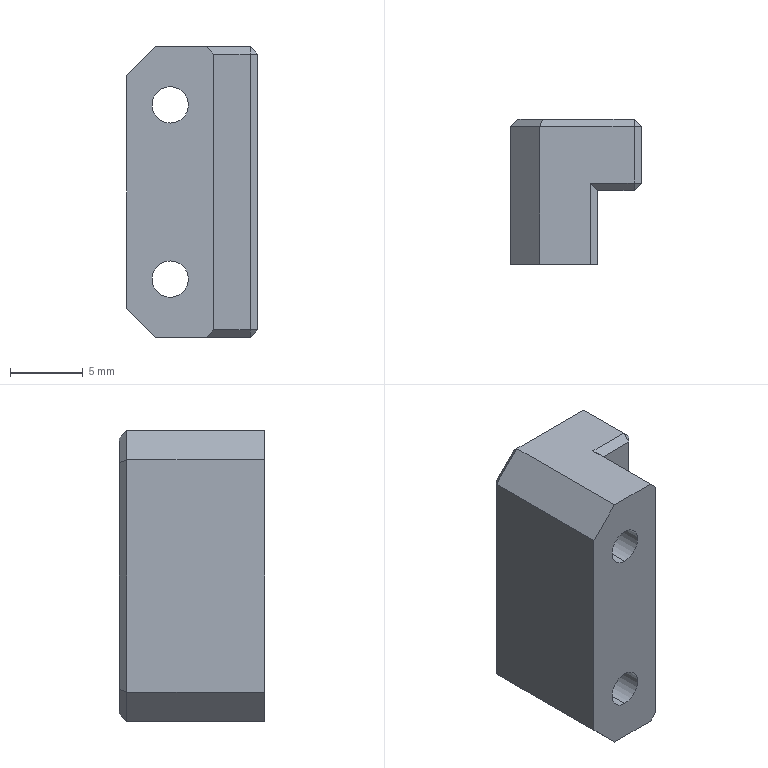Part | SolidWorks | features Chamfer 2, Extrusion 1, HoleWzd 1 | 1 solid | 35 faces | box 9 x 10 x 20 mm | volume 1341 mm3 | plane 27 | cone 4 | cylinder 4 | commonest cylinder face diameters 2.5 x4
STEP:
#1=CARTESIAN_POINT('',(3.,9.5,14.75));
#2=VERTEX_POINT('',#1);
#3=CARTESIAN_POINT('',(3.,9.5,17.25));
#4=VERTEX_POINT('',#3);
#5=CARTESIAN_POINT('',(3.,9.5,16.));
#6=DIRECTION('',(0.,1.,0.));
#7=DIRECTION('',(0.,0.,-1.));
#8=AXIS2_PLACEMENT_3D('',#5,#6,#7);
#9=CIRCLE('',#8,1.25);
#10=EDGE_CURVE('',#2,#4,#9,.T.);
#11=ORIENTED_EDGE('',*,*,#10,.F.);
#12=CARTESIAN_POINT('',(3.,10.,14.25));
#13=VERTEX_POINT('',#12);
#14=CARTESIAN_POINT('',(3.,9.5,14.75));
#15=DIRECTION('',(0.,0.7071,-0.7071));
#16=VECTOR('',#15,1000.);
#17=LINE('',#14,#16);
#18=EDGE_CURVE('',#2,#13,#17,.T.);
#19=ORIENTED_EDGE('',*,*,#18,.T.);
#20=CARTESIAN_POINT('',(3.,10.,17.75));
#21=VERTEX_POINT('',#20);
#22=CARTESIAN_POINT('',(3.,10.,16.));
#23=DIRECTION('',(0.,-1.,0.));
#24=DIRECTION('',(1.,0.,0.));
#25=AXIS2_PLACEMENT_3D('',#22,#23,#24);
#26=CIRCLE('',#25,1.75);
#27=EDGE_CURVE('',#21,#13,#26,.T.);
#28=ORIENTED_EDGE('',*,*,#27,.F.);
#29=CARTESIAN_POINT('',(3.,9.5,17.25));
#30=DIRECTION('',(0.,0.7071,0.7071));
#31=VECTOR('',#30,1000.);
#32=LINE('',#29,#31);
#33=EDGE_CURVE('',#4,#21,#32,.T.);
#34=ORIENTED_EDGE('',*,*,#33,.F.);
#35=EDGE_LOOP('',(#11,#19,#28,#34));
#36=FACE_OUTER_BOUND('',#35,.T.);
#37=CARTESIAN_POINT('',(3.,9.5,16.));
#38=DIRECTION('',(0.,1.,0.));
#39=DIRECTION('',(0.,0.,1.));
#40=AXIS2_PLACEMENT_3D('',#37,#38,#39);
#41=CONICAL_SURFACE('',#40,1.25,0.7854);
#42=ADVANCED_FACE('',(#36),#41,.F.);
#43=CARTESIAN_POINT('',(3.,9.5,2.75));
#44=VERTEX_POINT('',#43);
#45=CARTESIAN_POINT('',(3.,9.5,5.25));
#46=VERTEX_POINT('',#45);
#47=CARTESIAN_POINT('',(3.,9.5,4.));
#48=DIRECTION('',(0.,1.,0.));
#49=DIRECTION('',(0.,0.,-1.));
#50=AXIS2_PLACEMENT_3D('',#47,#48,#49);
#51=CIRCLE('',#50,1.25);
#52=EDGE_CURVE('',#44,#46,#51,.T.);
#53=ORIENTED_EDGE('',*,*,#52,.F.);
#54=CARTESIAN_POINT('',(3.,10.,2.25));
#55=VERTEX_POINT('',#54);
#56=CARTESIAN_POINT('',(3.,9.5,2.75));
#57=DIRECTION('',(0.,0.7071,-0.7071));
#58=VECTOR('',#57,1000.);
#59=LINE('',#56,#58);
#60=EDGE_CURVE('',#44,#55,#59,.T.);
#61=ORIENTED_EDGE('',*,*,#60,.T.);
#62=CARTESIAN_POINT('',(3.,10.,5.75));
#63=VERTEX_POINT('',#62);
#64=CARTESIAN_POINT('',(3.,10.,4.));
#65=DIRECTION('',(0.,-1.,0.));
#66=DIRECTION('',(1.,0.,0.));
#67=AXIS2_PLACEMENT_3D('',#64,#65,#66);
#68=CIRCLE('',#67,1.75);
#69=EDGE_CURVE('',#63,#55,#68,.T.);
#70=ORIENTED_EDGE('',*,*,#69,.F.);
#71=CARTESIAN_POINT('',(3.,9.5,5.25));
#72=DIRECTION('',(0.,0.7071,0.7071));
#73=VECTOR('',#72,1000.);
#74=LINE('',#71,#73);
#75=EDGE_CURVE('',#46,#63,#74,.T.);
#76=ORIENTED_EDGE('',*,*,#75,.F.);
#77=EDGE_LOOP('',(#53,#61,#70,#76));
#78=FACE_OUTER_BOUND('',#77,.T.);
#79=CARTESIAN_POINT('',(3.,9.5,4.));
#80=DIRECTION('',(0.,1.,0.));
#81=DIRECTION('',(0.,0.,1.));
#82=AXIS2_PLACEMENT_3D('',#79,#80,#81);
#83=CONICAL_SURFACE('',#82,1.25,0.7854);
#84=ADVANCED_FACE('',(#78),#83,.F.);
#85=CARTESIAN_POINT('',(3.,0.,14.75));
#86=VERTEX_POINT('',#85);
#87=CARTESIAN_POINT('',(3.,0.,17.25));
#88=VERTEX_POINT('',#87);
#89=CARTESIAN_POINT('',(3.,0.,16.));
#90=DIRECTION('',(0.,1.,0.));
#91=DIRECTION('',(0.,0.,1.));
#92=AXIS2_PLACEMENT_3D('',#89,#90,#91);
#93=CIRCLE('',#92,1.25);
#94=EDGE_CURVE('',#86,#88,#93,.T.);
#95=ORIENTED_EDGE('',*,*,#94,.F.);
#96=CARTESIAN_POINT('',(3.,10.,14.75));
#97=DIRECTION('',(0.,1.,0.));
#98=VECTOR('',#97,1000.);
#99=LINE('',#96,#98);
#100=EDGE_CURVE('',#86,#2,#99,.T.);
#101=ORIENTED_EDGE('',*,*,#100,.T.);
#102=ORIENTED_EDGE('',*,*,#10,.T.);
#103=CARTESIAN_POINT('',(3.,10.,17.25));
#104=DIRECTION('',(0.,1.,0.));
#105=VECTOR('',#104,1000.);
#106=LINE('',#103,#105);
#107=EDGE_CURVE('',#88,#4,#106,.T.);
#108=ORIENTED_EDGE('',*,*,#107,.F.);
#109=EDGE_LOOP('',(#95,#101,#102,#108));
#110=FACE_OUTER_BOUND('',#109,.T.);
#111=CARTESIAN_POINT('',(3.,10.,16.));
#112=DIRECTION('',(0.,1.,0.));
#113=DIRECTION('',(0.,0.,1.));
#114=AXIS2_PLACEMENT_3D('',#111,#112,#113);
#115=CYLINDRICAL_SURFACE('',#114,1.25);
#116=ADVANCED_FACE('',(#110),#115,.F.);
#117=CARTESIAN_POINT('',(3.,0.,2.75));
#118=VERTEX_POINT('',#117);
#119=CARTESIAN_POINT('',(3.,0.,5.25));
#120=VERTEX_POINT('',#119);
#121=CARTESIAN_POINT('',(3.,0.,4.));
#122=DIRECTION('',(0.,1.,0.));
#123=DIRECTION('',(0.,0.,1.));
#124=AXIS2_PLACEMENT_3D('',#121,#122,#123);
#125=CIRCLE('',#124,1.25);
#126=EDGE_CURVE('',#118,#120,#125,.T.);
#127=ORIENTED_EDGE('',*,*,#126,.F.);
#128=CARTESIAN_POINT('',(3.,10.,2.75));
#129=DIRECTION('',(0.,1.,0.));
#130=VECTOR('',#129,1000.);
#131=LINE('',#128,#130);
#132=EDGE_CURVE('',#118,#44,#131,.T.);
#133=ORIENTED_EDGE('',*,*,#132,.T.);
#134=ORIENTED_EDGE('',*,*,#52,.T.);
#135=CARTESIAN_POINT('',(3.,10.,5.25));
#136=DIRECTION('',(0.,1.,0.));
#137=VECTOR('',#136,1000.);
#138=LINE('',#135,#137);
#139=EDGE_CURVE('',#120,#46,#138,.T.);
#140=ORIENTED_EDGE('',*,*,#139,.F.);
#141=EDGE_LOOP('',(#127,#133,#134,#140));
#142=FACE_OUTER_BOUND('',#141,.T.);
#143=CARTESIAN_POINT('',(3.,10.,4.));
#144=DIRECTION('',(0.,1.,0.));
#145=DIRECTION('',(0.,0.,1.));
#146=AXIS2_PLACEMENT_3D('',#143,#144,#145);
#147=CYLINDRICAL_SURFACE('',#146,1.25);
#148=ADVANCED_FACE('',(#142),#147,.F.);
#149=CARTESIAN_POINT('',(0.,0.,18.));
#150=VERTEX_POINT('',#149);
#151=CARTESIAN_POINT('',(0.,9.5,18.));
#152=VERTEX_POINT('',#151);
#153=CARTESIAN_POINT('',(0.,10.,18.));
#154=DIRECTION('',(0.,1.,0.));
#155=VECTOR('',#154,1000.);
#156=LINE('',#153,#155);
#157=EDGE_CURVE('',#150,#152,#156,.T.);
#158=ORIENTED_EDGE('',*,*,#157,.T.);
#159=CARTESIAN_POINT('',(0.,9.5,2.));
#160=VERTEX_POINT('',#159);
#161=CARTESIAN_POINT('',(0.,9.5,20.));
#162=DIRECTION('',(0.,0.,-1.));
#163=VECTOR('',#162,1000.);
#164=LINE('',#161,#163);
#165=EDGE_CURVE('',#152,#160,#164,.T.);
#166=ORIENTED_EDGE('',*,*,#165,.T.);
#167=CARTESIAN_POINT('',(0.,0.,2.));
#168=VERTEX_POINT('',#167);
#169=CARTESIAN_POINT('',(0.,10.,2.));
#170=DIRECTION('',(0.,-1.,0.));
#171=VECTOR('',#170,1000.);
#172=LINE('',#169,#171);
#173=EDGE_CURVE('',#160,#168,#172,.T.);
#174=ORIENTED_EDGE('',*,*,#173,.T.);
#175=CARTESIAN_POINT('',(0.,0.,20.));
#176=DIRECTION('',(0.,0.,-1.));
#177=VECTOR('',#176,1000.);
#178=LINE('',#175,#177);
#179=EDGE_CURVE('',#150,#168,#178,.T.);
#180=ORIENTED_EDGE('',*,*,#179,.F.);
#181=EDGE_LOOP('',(#158,#166,#174,#180));
#182=FACE_OUTER_BOUND('',#181,.T.);
#183=CARTESIAN_POINT('',(0.,10.,20.));
#184=DIRECTION('',(1.,0.,0.));
#185=DIRECTION('',(0.,1.,0.));
#186=AXIS2_PLACEMENT_3D('',#183,#184,#185);
#187=PLANE('',#186);
#188=ADVANCED_FACE('',(#182),#187,.F.);
#189=CARTESIAN_POINT('',(3.,0.,16.));
#190=DIRECTION('',(0.,1.,0.));
#191=DIRECTION('',(0.,0.,1.));
#192=AXIS2_PLACEMENT_3D('',#189,#190,#191);
#193=CIRCLE('',#192,1.25);
#194=EDGE_CURVE('',#88,#86,#193,.T.);
#195=ORIENTED_EDGE('',*,*,#194,.T.);
#196=ORIENTED_EDGE('',*,*,#94,.T.);
#197=EDGE_LOOP('',(#195,#196));
#198=FACE_BOUND('',#197,.T.);
#199=CARTESIAN_POINT('',(3.,0.,4.));
#200=DIRECTION('',(0.,1.,0.));
#201=DIRECTION('',(0.,0.,1.));
#202=AXIS2_PLACEMENT_3D('',#199,#200,#201);
#203=CIRCLE('',#202,1.25);
#204=EDGE_CURVE('',#120,#118,#203,.T.);
#205=ORIENTED_EDGE('',*,*,#204,.T.);
#206=ORIENTED_EDGE('',*,*,#126,.T.);
#207=EDGE_LOOP('',(#205,#206));
#208=FACE_BOUND('',#207,.T.);
#209=CARTESIAN_POINT('',(6.,0.,19.5));
#210=VERTEX_POINT('',#209);
#211=CARTESIAN_POINT('',(6.,0.,0.5));
#212=VERTEX_POINT('',#211);
#213=CARTESIAN_POINT('',(6.,0.,20.));
#214=DIRECTION('',(0.,0.,-1.));
#215=VECTOR('',#214,1000.);
#216=LINE('',#213,#215);
#217=EDGE_CURVE('',#210,#212,#216,.T.);
#218=ORIENTED_EDGE('',*,*,#217,.F.);
#219=CARTESIAN_POINT('',(5.5,0.,20.));
#220=VERTEX_POINT('',#219);
#221=CARTESIAN_POINT('',(5.5,0.,20.));
#222=DIRECTION('',(-0.7071,0.,0.7071));
#223=VECTOR('',#222,1000.);
#224=LINE('',#221,#223);
#225=EDGE_CURVE('',#210,#220,#224,.T.);
#226=ORIENTED_EDGE('',*,*,#225,.T.);
#227=CARTESIAN_POINT('',(2.,0.,20.));
#228=VERTEX_POINT('',#227);
#229=CARTESIAN_POINT('',(0.,0.,20.));
#230=DIRECTION('',(1.,0.,0.));
#231=VECTOR('',#230,1000.);
#232=LINE('',#229,#231);
#233=EDGE_CURVE('',#228,#220,#232,.T.);
#234=ORIENTED_EDGE('',*,*,#233,.F.);
#235=CARTESIAN_POINT('',(2.,0.,20.));
#236=DIRECTION('',(-0.7071,0.,-0.7071));
#237=VECTOR('',#236,1000.);
#238=LINE('',#235,#237);
#239=EDGE_CURVE('',#228,#150,#238,.T.);
#240=ORIENTED_EDGE('',*,*,#239,.T.);
#241=ORIENTED_EDGE('',*,*,#179,.T.);
#242=CARTESIAN_POINT('',(2.,0.,0.));
#243=VERTEX_POINT('',#242);
#244=CARTESIAN_POINT('',(0.,0.,2.));
#245=DIRECTION('',(0.7071,0.,-0.7071));
#246=VECTOR('',#245,1000.);
#247=LINE('',#244,#246);
#248=EDGE_CURVE('',#168,#243,#247,.T.);
#249=ORIENTED_EDGE('',*,*,#248,.T.);
#250=CARTESIAN_POINT('',(5.5,0.,0.));
#251=VERTEX_POINT('',#250);
#252=CARTESIAN_POINT('',(0.,0.,0.));
#253=DIRECTION('',(1.,0.,0.));
#254=VECTOR('',#253,1000.);
#255=LINE('',#252,#254);
#256=EDGE_CURVE('',#243,#251,#255,.T.);
#257=ORIENTED_EDGE('',*,*,#256,.T.);
#258=CARTESIAN_POINT('',(6.,0.,0.5));
#259=DIRECTION('',(0.7071,0.,0.7071));
#260=VECTOR('',#259,1000.);
#261=LINE('',#258,#260);
#262=EDGE_CURVE('',#251,#212,#261,.T.);
#263=ORIENTED_EDGE('',*,*,#262,.T.);
#264=EDGE_LOOP('',(#218,#226,#234,#240,#241,#249,#257,#263));
#265=FACE_OUTER_BOUND('',#264,.T.);
#266=CARTESIAN_POINT('',(0.,0.,20.));
#267=DIRECTION('',(0.,1.,0.));
#268=DIRECTION('',(0.,0.,1.));
#269=AXIS2_PLACEMENT_3D('',#266,#267,#268);
#270=PLANE('',#269);
#271=ADVANCED_FACE('',(#198,#208,#265),#270,.F.);
#272=CARTESIAN_POINT('',(6.,5.1,19.5));
#273=VERTEX_POINT('',#272);
#274=CARTESIAN_POINT('',(6.,5.1,0.5));
#275=VERTEX_POINT('',#274);
#276=CARTESIAN_POINT('',(6.,5.1,20.));
#277=DIRECTION('',(0.,0.,-1.));
#278=VECTOR('',#277,1000.);
#279=LINE('',#276,#278);
#280=EDGE_CURVE('',#273,#275,#279,.T.);
#281=ORIENTED_EDGE('',*,*,#280,.F.);
#282=CARTESIAN_POINT('',(6.,0.,19.5));
#283=DIRECTION('',(0.,-1.,0.));
#284=VECTOR('',#283,1000.);
#285=LINE('',#282,#284);
#286=EDGE_CURVE('',#273,#210,#285,.T.);
#287=ORIENTED_EDGE('',*,*,#286,.T.);
#288=ORIENTED_EDGE('',*,*,#217,.T.);
#289=CARTESIAN_POINT('',(6.,0.,0.5));
#290=DIRECTION('',(0.,1.,0.));
#291=VECTOR('',#290,1000.);
#292=LINE('',#289,#291);
#293=EDGE_CURVE('',#212,#275,#292,.T.);
#294=ORIENTED_EDGE('',*,*,#293,.T.);
#295=EDGE_LOOP('',(#281,#287,#288,#294));
#296=FACE_OUTER_BOUND('',#295,.T.);
#297=CARTESIAN_POINT('',(6.,0.,20.));
#298=DIRECTION('',(-1.,0.,0.));
#299=DIRECTION('',(0.,0.,1.));
#300=AXIS2_PLACEMENT_3D('',#297,#298,#299);
#301=PLANE('',#300);
#302=ADVANCED_FACE('',(#296),#301,.F.);
#303=CARTESIAN_POINT('',(8.5,5.1,0.5));
#304=VERTEX_POINT('',#303);
#305=CARTESIAN_POINT('',(8.5,5.1,19.5));
#306=VERTEX_POINT('',#305);
#307=CARTESIAN_POINT('',(8.5,5.1,20.));
#308=DIRECTION('',(0.,0.,1.));
#309=VECTOR('',#308,1000.);
#310=LINE('',#307,#309);
#311=EDGE_CURVE('',#304,#306,#310,.T.);
#312=ORIENTED_EDGE('',*,*,#311,.T.);
#313=CARTESIAN_POINT('',(6.,5.1,19.5));
#314=DIRECTION('',(-1.,0.,0.));
#315=VECTOR('',#314,1000.);
#316=LINE('',#313,#315);
#317=EDGE_CURVE('',#306,#273,#316,.T.);
#318=ORIENTED_EDGE('',*,*,#317,.T.);
#319=ORIENTED_EDGE('',*,*,#280,.T.);
#320=CARTESIAN_POINT('',(6.,5.1,0.5));
#321=DIRECTION('',(1.,0.,0.));
#322=VECTOR('',#321,1000.);
#323=LINE('',#320,#322);
#324=EDGE_CURVE('',#275,#304,#323,.T.);
#325=ORIENTED_EDGE('',*,*,#324,.T.);
#326=EDGE_LOOP('',(#312,#318,#319,#325));
#327=FACE_OUTER_BOUND('',#326,.T.);
#328=CARTESIAN_POINT('',(6.,5.1,20.));
#329=DIRECTION('',(0.,1.,0.));
#330=DIRECTION('',(0.,0.,1.));
#331=AXIS2_PLACEMENT_3D('',#328,#329,#330);
#332=PLANE('',#331);
#333=ADVANCED_FACE('',(#327),#332,.F.);
#334=CARTESIAN_POINT('',(9.,5.6,0.5));
#335=VERTEX_POINT('',#334);
#336=CARTESIAN_POINT('',(9.,9.5,0.5));
#337=VERTEX_POINT('',#336);
#338=CARTESIAN_POINT('',(9.,5.1,0.5));
#339=DIRECTION('',(0.,1.,0.));
#340=VECTOR('',#339,1000.);
#341=LINE('',#338,#340);
#342=EDGE_CURVE('',#335,#337,#341,.T.);
#343=ORIENTED_EDGE('',*,*,#342,.T.);
#344=CARTESIAN_POINT('',(9.,9.5,19.5));
#345=VERTEX_POINT('',#344);
#346=CARTESIAN_POINT('',(9.,9.5,20.));
#347=DIRECTION('',(0.,0.,1.));
#348=VECTOR('',#347,1000.);
#349=LINE('',#346,#348);
#350=EDGE_CURVE('',#337,#345,#349,.T.);
#351=ORIENTED_EDGE('',*,*,#350,.T.);
#352=CARTESIAN_POINT('',(9.,5.6,19.5));
#353=VERTEX_POINT('',#352);
#354=CARTESIAN_POINT('',(9.,5.1,19.5));
#355=DIRECTION('',(0.,-1.,0.));
#356=VECTOR('',#355,1000.);
#357=LINE('',#354,#356);
#358=EDGE_CURVE('',#345,#353,#357,.T.);
#359=ORIENTED_EDGE('',*,*,#358,.T.);
#360=CARTESIAN_POINT('',(9.,5.6,20.));
#361=DIRECTION('',(0.,0.,-1.));
#362=VECTOR('',#361,1000.);
#363=LINE('',#360,#362);
#364=EDGE_CURVE('',#353,#335,#363,.T.);
#365=ORIENTED_EDGE('',*,*,#364,.T.);
#366=EDGE_LOOP('',(#343,#351,#359,#365));
#367=FACE_OUTER_BOUND('',#366,.T.);
#368=CARTESIAN_POINT('',(9.,5.1,20.));
#369=DIRECTION('',(-1.,0.,0.));
#370=DIRECTION('',(0.,0.,1.));
#371=AXIS2_PLACEMENT_3D('',#368,#369,#370);
#372=PLANE('',#371);
#373=ADVANCED_FACE('',(#367),#372,.F.);
#374=ORIENTED_EDGE('',*,*,#69,.T.);
#375=CARTESIAN_POINT('',(3.,10.,4.));
#376=DIRECTION('',(0.,-1.,0.));
#377=DIRECTION('',(1.,0.,0.));
#378=AXIS2_PLACEMENT_3D('',#375,#376,#377);
#379=CIRCLE('',#378,1.75);
#380=EDGE_CURVE('',#55,#63,#379,.T.);
#381=ORIENTED_EDGE('',*,*,#380,.T.);
#382=EDGE_LOOP('',(#374,#381));
#383=FACE_BOUND('',#382,.T.);
#384=ORIENTED_EDGE('',*,*,#27,.T.);
#385=CARTESIAN_POINT('',(3.,10.,16.));
#386=DIRECTION('',(0.,-1.,0.));
#387=DIRECTION('',(1.,0.,0.));
#388=AXIS2_PLACEMENT_3D('',#385,#386,#387);
#389=CIRCLE('',#388,1.75);
#390=EDGE_CURVE('',#13,#21,#389,.T.);
#391=ORIENTED_EDGE('',*,*,#390,.T.);
#392=EDGE_LOOP('',(#384,#391));
#393=FACE_BOUND('',#392,.T.);
#394=CARTESIAN_POINT('',(2.207,10.,19.5));
#395=VERTEX_POINT('',#394);
#396=CARTESIAN_POINT('',(8.5,10.,19.5));
#397=VERTEX_POINT('',#396);
#398=CARTESIAN_POINT('',(9.,10.,19.5));
#399=DIRECTION('',(1.,0.,0.));
#400=VECTOR('',#399,1000.);
#401=LINE('',#398,#400);
#402=EDGE_CURVE('',#395,#397,#401,.T.);
#403=ORIENTED_EDGE('',*,*,#402,.T.);
#404=CARTESIAN_POINT('',(8.5,10.,0.5));
#405=VERTEX_POINT('',#404);
#406=CARTESIAN_POINT('',(8.5,10.,20.));
#407=DIRECTION('',(0.,0.,-1.));
#408=VECTOR('',#407,1000.);
#409=LINE('',#406,#408);
#410=EDGE_CURVE('',#397,#405,#409,.T.);
#411=ORIENTED_EDGE('',*,*,#410,.T.);
#412=CARTESIAN_POINT('',(2.207,10.,0.5));
#413=VERTEX_POINT('',#412);
#414=CARTESIAN_POINT('',(9.,10.,0.5));
#415=DIRECTION('',(-1.,0.,0.));
#416=VECTOR('',#415,1000.);
#417=LINE('',#414,#416);
#418=EDGE_CURVE('',#405,#413,#417,.T.);
#419=ORIENTED_EDGE('',*,*,#418,.T.);
#420=CARTESIAN_POINT('',(0.5,10.,2.207));
#421=VERTEX_POINT('',#420);
#422=CARTESIAN_POINT('',(0.3536,10.,2.354));
#423=DIRECTION('',(-0.7071,0.,0.7071));
#424=VECTOR('',#423,1000.);
#425=LINE('',#422,#424);
#426=EDGE_CURVE('',#413,#421,#425,.T.);
#427=ORIENTED_EDGE('',*,*,#426,.T.);
#428=CARTESIAN_POINT('',(0.5,10.,17.793));
#429=VERTEX_POINT('',#428);
#430=CARTESIAN_POINT('',(0.5,10.,20.));
#431=DIRECTION('',(0.,0.,1.));
#432=VECTOR('',#431,1000.);
#433=LINE('',#430,#432);
#434=EDGE_CURVE('',#421,#429,#433,.T.);
#435=ORIENTED_EDGE('',*,*,#434,.T.);
#436=CARTESIAN_POINT('',(2.354,10.,19.646));
#437=DIRECTION('',(0.7071,0.,0.7071));
#438=VECTOR('',#437,1000.);
#439=LINE('',#436,#438);
#440=EDGE_CURVE('',#429,#395,#439,.T.);
#441=ORIENTED_EDGE('',*,*,#440,.T.);
#442=EDGE_LOOP('',(#403,#411,#419,#427,#435,#441));
#443=FACE_OUTER_BOUND('',#442,.T.);
#444=CARTESIAN_POINT('',(9.,10.,20.));
#445=DIRECTION('',(0.,-1.,0.));
#446=DIRECTION('',(1.,0.,0.));
#447=AXIS2_PLACEMENT_3D('',#444,#445,#446);
#448=PLANE('',#447);
#449=ADVANCED_FACE('',(#383,#393,#443),#448,.F.);
#450=CARTESIAN_POINT('',(8.5,5.6,20.));
#451=VERTEX_POINT('',#450);
#452=CARTESIAN_POINT('',(8.5,9.5,20.));
#453=VERTEX_POINT('',#452);
#454=CARTESIAN_POINT('',(8.5,10.,20.));
#455=DIRECTION('',(0.,1.,0.));
#456=VECTOR('',#455,1000.);
#457=LINE('',#454,#456);
#458=EDGE_CURVE('',#451,#453,#457,.T.);
#459=ORIENTED_EDGE('',*,*,#458,.T.);
#460=CARTESIAN_POINT('',(2.,9.5,20.));
#461=VERTEX_POINT('',#460);
#462=CARTESIAN_POINT('',(2.,9.5,20.));
#463=DIRECTION('',(-1.,0.,0.));
#464=VECTOR('',#463,1000.);
#465=LINE('',#462,#464);
#466=EDGE_CURVE('',#453,#461,#465,.T.);
#467=ORIENTED_EDGE('',*,*,#466,.T.);
#468=CARTESIAN_POINT('',(2.,0.,20.));
#469=DIRECTION('',(0.,-1.,0.));
#470=VECTOR('',#469,1000.);
#471=LINE('',#468,#470);
#472=EDGE_CURVE('',#461,#228,#471,.T.);
#473=ORIENTED_EDGE('',*,*,#472,.T.);
#474=ORIENTED_EDGE('',*,*,#233,.T.);
#475=CARTESIAN_POINT('',(5.5,5.6,20.));
#476=VERTEX_POINT('',#475);
#477=CARTESIAN_POINT('',(5.5,5.1,20.));
#478=DIRECTION('',(0.,1.,0.));
#479=VECTOR('',#478,1000.);
#480=LINE('',#477,#479);
#481=EDGE_CURVE('',#220,#476,#480,.T.);
#482=ORIENTED_EDGE('',*,*,#481,.T.);
#483=CARTESIAN_POINT('',(9.,5.6,20.));
#484=DIRECTION('',(1.,0.,0.));
#485=VECTOR('',#484,1000.);
#486=LINE('',#483,#485);
#487=EDGE_CURVE('',#476,#451,#486,.T.);
#488=ORIENTED_EDGE('',*,*,#487,.T.);
#489=EDGE_LOOP('',(#459,#467,#473,#474,#482,#488));
#490=FACE_OUTER_BOUND('',#489,.T.);
#491=CARTESIAN_POINT('',(0.,0.,20.));
#492=DIRECTION('',(0.,0.,1.));
#493=DIRECTION('',(1.,0.,0.));
#494=AXIS2_PLACEMENT_3D('',#491,#492,#493);
#495=PLANE('',#494);
#496=ADVANCED_FACE('',(#490),#495,.T.);
#497=CARTESIAN_POINT('',(2.,9.5,0.));
#498=VERTEX_POINT('',#497);
#499=CARTESIAN_POINT('',(2.,0.,0.));
#500=DIRECTION('',(0.,1.,0.));
#501=VECTOR('',#500,1000.);
#502=LINE('',#499,#501);
#503=EDGE_CURVE('',#243,#498,#502,.T.);
#504=ORIENTED_EDGE('',*,*,#503,.T.);
#505=CARTESIAN_POINT('',(8.5,9.5,0.));
#506=VERTEX_POINT('',#505);
#507=CARTESIAN_POINT('',(0.,9.5,0.));
#508=DIRECTION('',(1.,0.,0.));
#509=VECTOR('',#508,1000.);
#510=LINE('',#507,#509);
#511=EDGE_CURVE('',#498,#506,#510,.T.);
#512=ORIENTED_EDGE('',*,*,#511,.T.);
#513=CARTESIAN_POINT('',(8.5,5.6,0.));
#514=VERTEX_POINT('',#513);
#515=CARTESIAN_POINT('',(8.5,0.,0.));
#516=DIRECTION('',(0.,-1.,0.));
#517=VECTOR('',#516,1000.);
#518=LINE('',#515,#517);
#519=EDGE_CURVE('',#506,#514,#518,.T.);
#520=ORIENTED_EDGE('',*,*,#519,.T.);
#521=CARTESIAN_POINT('',(5.5,5.6,0.));
#522=VERTEX_POINT('',#521);
#523=CARTESIAN_POINT('',(0.,5.6,0.));
#524=DIRECTION('',(-1.,0.,0.));
#525=VECTOR('',#524,1000.);
#526=LINE('',#523,#525);
#527=EDGE_CURVE('',#514,#522,#526,.T.);
#528=ORIENTED_EDGE('',*,*,#527,.T.);
#529=CARTESIAN_POINT('',(5.5,0.,0.));
#530=DIRECTION('',(0.,-1.,0.));
#531=VECTOR('',#530,1000.);
#532=LINE('',#529,#531);
#533=EDGE_CURVE('',#522,#251,#532,.T.);
#534=ORIENTED_EDGE('',*,*,#533,.T.);
#535=ORIENTED_EDGE('',*,*,#256,.F.);
#536=EDGE_LOOP('',(#504,#512,#520,#528,#534,#535));
#537=FACE_OUTER_BOUND('',#536,.T.);
#538=CARTESIAN_POINT('',(0.,0.,0.));
#539=DIRECTION('',(0.,0.,1.));
#540=DIRECTION('',(1.,0.,0.));
#541=AXIS2_PLACEMENT_3D('',#538,#539,#540);
#542=PLANE('',#541);
#543=ADVANCED_FACE('',(#537),#542,.F.);
#544=ORIENTED_EDGE('',*,*,#132,.F.);
#545=ORIENTED_EDGE('',*,*,#204,.F.);
#546=ORIENTED_EDGE('',*,*,#139,.T.);
#547=CARTESIAN_POINT('',(3.,9.5,4.));
#548=DIRECTION('',(0.,1.,0.));
#549=DIRECTION('',(0.,0.,-1.));
#550=AXIS2_PLACEMENT_3D('',#547,#548,#549);
#551=CIRCLE('',#550,1.25);
#552=EDGE_CURVE('',#46,#44,#551,.T.);
#553=ORIENTED_EDGE('',*,*,#552,.T.);
#554=EDGE_LOOP('',(#544,#545,#546,#553));
#555=FACE_OUTER_BOUND('',#554,.T.);
#556=CARTESIAN_POINT('',(3.,10.,4.));
#557=DIRECTION('',(0.,1.,0.));
#558=DIRECTION('',(0.,0.,1.));
#559=AXIS2_PLACEMENT_3D('',#556,#557,#558);
#560=CYLINDRICAL_SURFACE('',#559,1.25);
#561=ADVANCED_FACE('',(#555),#560,.F.);
#562=ORIENTED_EDGE('',*,*,#100,.F.);
#563=ORIENTED_EDGE('',*,*,#194,.F.);
#564=ORIENTED_EDGE('',*,*,#107,.T.);
#565=CARTESIAN_POINT('',(3.,9.5,16.));
#566=DIRECTION('',(0.,1.,0.));
#567=DIRECTION('',(0.,0.,-1.));
#568=AXIS2_PLACEMENT_3D('',#565,#566,#567);
#569=CIRCLE('',#568,1.25);
#570=EDGE_CURVE('',#4,#2,#569,.T.);
#571=ORIENTED_EDGE('',*,*,#570,.T.);
#572=EDGE_LOOP('',(#562,#563,#564,#571));
#573=FACE_OUTER_BOUND('',#572,.T.);
#574=CARTESIAN_POINT('',(3.,10.,16.));
#575=DIRECTION('',(0.,1.,0.));
#576=DIRECTION('',(0.,0.,1.));
#577=AXIS2_PLACEMENT_3D('',#574,#575,#576);
#578=CYLINDRICAL_SURFACE('',#577,1.25);
#579=ADVANCED_FACE('',(#573),#578,.F.);
#580=ORIENTED_EDGE('',*,*,#173,.F.);
#581=CARTESIAN_POINT('',(2.,9.5,0.));
#582=DIRECTION('',(0.7071,0.,-0.7071));
#583=VECTOR('',#582,1000.);
#584=LINE('',#581,#583);
#585=EDGE_CURVE('',#160,#498,#584,.T.);
#586=ORIENTED_EDGE('',*,*,#585,.T.);
#587=ORIENTED_EDGE('',*,*,#503,.F.);
#588=ORIENTED_EDGE('',*,*,#248,.F.);
#589=EDGE_LOOP('',(#580,#586,#587,#588));
#590=FACE_OUTER_BOUND('',#589,.T.);
#591=CARTESIAN_POINT('',(0.,10.,2.));
#592=DIRECTION('',(0.7071,0.,0.7071));
#593=DIRECTION('',(0.,-1.,0.));
#594=AXIS2_PLACEMENT_3D('',#591,#592,#593);
#595=PLANE('',#594);
#596=ADVANCED_FACE('',(#590),#595,.F.);
#597=ORIENTED_EDGE('',*,*,#472,.F.);
#598=CARTESIAN_POINT('',(0.,9.5,18.));
#599=DIRECTION('',(-0.7071,0.,-0.7071));
#600=VECTOR('',#599,1000.);
#601=LINE('',#598,#600);
#602=EDGE_CURVE('',#461,#152,#601,.T.);
#603=ORIENTED_EDGE('',*,*,#602,.T.);
#604=ORIENTED_EDGE('',*,*,#157,.F.);
#605=ORIENTED_EDGE('',*,*,#239,.F.);
#606=EDGE_LOOP('',(#597,#603,#604,#605));
#607=FACE_OUTER_BOUND('',#606,.T.);
#608=CARTESIAN_POINT('',(2.,0.,20.));
#609=DIRECTION('',(-0.7071,0.,0.7071));
#610=DIRECTION('',(0.,1.,0.));
#611=AXIS2_PLACEMENT_3D('',#608,#609,#610);
#612=PLANE('',#611);
#613=ADVANCED_FACE('',(#607),#612,.T.);
#614=ORIENTED_EDGE('',*,*,#60,.F.);
#615=ORIENTED_EDGE('',*,*,#552,.F.);
#616=ORIENTED_EDGE('',*,*,#75,.T.);
#617=ORIENTED_EDGE('',*,*,#380,.F.);
#618=EDGE_LOOP('',(#614,#615,#616,#617));
#619=FACE_OUTER_BOUND('',#618,.T.);
#620=CARTESIAN_POINT('',(3.,9.5,4.));
#621=DIRECTION('',(0.,1.,0.));
#622=DIRECTION('',(0.,0.,1.));
#623=AXIS2_PLACEMENT_3D('',#620,#621,#622);
#624=CONICAL_SURFACE('',#623,1.25,0.7854);
#625=ADVANCED_FACE('',(#619),#624,.F.);
#626=ORIENTED_EDGE('',*,*,#18,.F.);
#627=ORIENTED_EDGE('',*,*,#570,.F.);
#628=ORIENTED_EDGE('',*,*,#33,.T.);
#629=ORIENTED_EDGE('',*,*,#390,.F.);
#630=EDGE_LOOP('',(#626,#627,#628,#629));
#631=FACE_OUTER_BOUND('',#630,.T.);
#632=CARTESIAN_POINT('',(3.,9.5,16.));
#633=DIRECTION('',(0.,1.,0.));
#634=DIRECTION('',(0.,0.,1.));
#635=AXIS2_PLACEMENT_3D('',#632,#633,#634);
#636=CONICAL_SURFACE('',#635,1.25,0.7854);
#637=ADVANCED_FACE('',(#631),#636,.F.);
#638=ORIENTED_EDGE('',*,*,#225,.F.);
#639=ORIENTED_EDGE('',*,*,#286,.F.);
#640=CARTESIAN_POINT('',(7.367,3.733,18.133));
#641=DIRECTION('',(0.5774,-0.5774,-0.5774));
#642=VECTOR('',#641,1000.);
#643=LINE('',#640,#642);
#644=EDGE_CURVE('',#476,#273,#643,.T.);
#645=ORIENTED_EDGE('',*,*,#644,.F.);
#646=ORIENTED_EDGE('',*,*,#481,.F.);
#647=EDGE_LOOP('',(#638,#639,#645,#646));
#648=FACE_OUTER_BOUND('',#647,.T.);
#649=CARTESIAN_POINT('',(5.5,0.,20.));
#650=DIRECTION('',(0.7071,0.,0.7071));
#651=DIRECTION('',(0.,-1.,0.));
#652=AXIS2_PLACEMENT_3D('',#649,#650,#651);
#653=PLANE('',#652);
#654=ADVANCED_FACE('',(#648),#653,.T.);
#655=ORIENTED_EDGE('',*,*,#262,.F.);
#656=ORIENTED_EDGE('',*,*,#533,.F.);
#657=CARTESIAN_POINT('',(6.,5.1,0.5));
#658=DIRECTION('',(-0.5774,0.5774,-0.5774));
#659=VECTOR('',#658,1000.);
#660=LINE('',#657,#659);
#661=EDGE_CURVE('',#275,#522,#660,.T.);
#662=ORIENTED_EDGE('',*,*,#661,.F.);
#663=ORIENTED_EDGE('',*,*,#293,.F.);
#664=EDGE_LOOP('',(#655,#656,#662,#663));
#665=FACE_OUTER_BOUND('',#664,.T.);
#666=CARTESIAN_POINT('',(6.,0.,0.5));
#667=DIRECTION('',(-0.7071,0.,0.7071));
#668=DIRECTION('',(0.,1.,0.));
#669=AXIS2_PLACEMENT_3D('',#666,#667,#668);
#670=PLANE('',#669);
#671=ADVANCED_FACE('',(#665),#670,.F.);
#672=ORIENTED_EDGE('',*,*,#644,.T.);
#673=ORIENTED_EDGE('',*,*,#317,.F.);
#674=CARTESIAN_POINT('',(8.5,5.35,19.75));
#675=DIRECTION('',(0.,-0.7071,-0.7071));
#676=VECTOR('',#675,1000.);
#677=LINE('',#674,#676);
#678=EDGE_CURVE('',#451,#306,#677,.T.);
#679=ORIENTED_EDGE('',*,*,#678,.F.);
#680=ORIENTED_EDGE('',*,*,#487,.F.);
#681=EDGE_LOOP('',(#672,#673,#679,#680));
#682=FACE_OUTER_BOUND('',#681,.T.);
#683=CARTESIAN_POINT('',(0.,5.6,20.));
#684=DIRECTION('',(0.,-0.7071,0.7071));
#685=DIRECTION('',(-1.,0.,0.));
#686=AXIS2_PLACEMENT_3D('',#683,#684,#685);
#687=PLANE('',#686);
#688=ADVANCED_FACE('',(#682),#687,.T.);
#689=CARTESIAN_POINT('',(-0.7534,8.747,1.688));
#690=DIRECTION('',(0.6786,0.6786,0.2811));
#691=VECTOR('',#690,1000.);
#692=LINE('',#689,#691);
#693=EDGE_CURVE('',#160,#421,#692,.T.);
#694=ORIENTED_EDGE('',*,*,#693,.F.);
#695=ORIENTED_EDGE('',*,*,#165,.F.);
#696=CARTESIAN_POINT('',(-0.3815,9.119,18.158));
#697=DIRECTION('',(-0.6786,-0.6786,0.2811));
#698=VECTOR('',#697,1000.);
#699=LINE('',#696,#698);
#700=EDGE_CURVE('',#429,#152,#699,.T.);
#701=ORIENTED_EDGE('',*,*,#700,.F.);
#702=ORIENTED_EDGE('',*,*,#434,.F.);
#703=EDGE_LOOP('',(#694,#695,#701,#702));
#704=FACE_OUTER_BOUND('',#703,.T.);
#705=CARTESIAN_POINT('',(0.,9.5,20.));
#706=DIRECTION('',(0.7071,-0.7071,0.));
#707=DIRECTION('',(0.,0.,-1.));
#708=AXIS2_PLACEMENT_3D('',#705,#706,#707);
#709=PLANE('',#708);
#710=ADVANCED_FACE('',(#704),#709,.F.);
#711=ORIENTED_EDGE('',*,*,#661,.T.);
#712=ORIENTED_EDGE('',*,*,#527,.F.);
#713=CARTESIAN_POINT('',(8.5,5.6,0.));
#714=DIRECTION('',(0.,0.7071,-0.7071));
#715=VECTOR('',#714,1000.);
#716=LINE('',#713,#715);
#717=EDGE_CURVE('',#304,#514,#716,.T.);
#718=ORIENTED_EDGE('',*,*,#717,.F.);
#719=ORIENTED_EDGE('',*,*,#324,.F.);
#720=EDGE_LOOP('',(#711,#712,#718,#719));
#721=FACE_OUTER_BOUND('',#720,.T.);
#722=CARTESIAN_POINT('',(6.,5.1,0.5));
#723=DIRECTION('',(0.,0.7071,0.7071));
#724=DIRECTION('',(1.,0.,0.));
#725=AXIS2_PLACEMENT_3D('',#722,#723,#724);
#726=PLANE('',#725);
#727=ADVANCED_FACE('',(#721),#726,.F.);
#728=CARTESIAN_POINT('',(9.,5.6,19.5));
#729=DIRECTION('',(0.7071,0.7071,0.));
#730=VECTOR('',#729,1000.);
#731=LINE('',#728,#730);
#732=EDGE_CURVE('',#306,#353,#731,.T.);
#733=ORIENTED_EDGE('',*,*,#732,.F.);
#734=ORIENTED_EDGE('',*,*,#311,.F.);
#735=CARTESIAN_POINT('',(8.75,5.35,0.5));
#736=DIRECTION('',(-0.7071,-0.7071,0.));
#737=VECTOR('',#736,1000.);
#738=LINE('',#735,#737);
#739=EDGE_CURVE('',#335,#304,#738,.T.);
#740=ORIENTED_EDGE('',*,*,#739,.F.);
#741=ORIENTED_EDGE('',*,*,#364,.F.);
#742=EDGE_LOOP('',(#733,#734,#740,#741));
#743=FACE_OUTER_BOUND('',#742,.T.);
#744=CARTESIAN_POINT('',(9.,5.6,20.));
#745=DIRECTION('',(-0.7071,0.7071,0.));
#746=DIRECTION('',(0.,0.,-1.));
#747=AXIS2_PLACEMENT_3D('',#744,#745,#746);
#748=PLANE('',#747);
#749=ADVANCED_FACE('',(#743),#748,.F.);
#750=ORIENTED_EDGE('',*,*,#678,.T.);
#751=ORIENTED_EDGE('',*,*,#732,.T.);
#752=CARTESIAN_POINT('',(9.,5.6,19.5));
#753=DIRECTION('',(0.7071,0.,-0.7071));
#754=VECTOR('',#753,1000.);
#755=LINE('',#752,#754);
#756=EDGE_CURVE('',#451,#353,#755,.T.);
#757=ORIENTED_EDGE('',*,*,#756,.F.);
#758=EDGE_LOOP('',(#750,#751,#757));
#759=FACE_OUTER_BOUND('',#758,.T.);
#760=CARTESIAN_POINT('',(9.,5.6,19.5));
#761=DIRECTION('',(0.5774,-0.5774,0.5774));
#762=DIRECTION('',(0.7071,0.,-0.7071));
#763=AXIS2_PLACEMENT_3D('',#760,#761,#762);
#764=PLANE('',#763);
#765=ADVANCED_FACE('',(#759),#764,.T.);
#766=ORIENTED_EDGE('',*,*,#700,.T.);
#767=ORIENTED_EDGE('',*,*,#602,.F.);
#768=CARTESIAN_POINT('',(1.8,9.016,20.484));
#769=DIRECTION('',(-0.2811,-0.6786,0.6786));
#770=VECTOR('',#769,1000.);
#771=LINE('',#768,#770);
#772=EDGE_CURVE('',#395,#461,#771,.T.);
#773=ORIENTED_EDGE('',*,*,#772,.F.);
#774=ORIENTED_EDGE('',*,*,#440,.F.);
#775=EDGE_LOOP('',(#766,#767,#773,#774));
#776=FACE_OUTER_BOUND('',#775,.T.);
#777=CARTESIAN_POINT('',(5.854,10.,23.146));
#778=DIRECTION('',(-0.5,0.7071,0.5));
#779=DIRECTION('',(-0.7071,0.,-0.7071));
#780=AXIS2_PLACEMENT_3D('',#777,#778,#779);
#781=PLANE('',#780);
#782=ADVANCED_FACE('',(#776),#781,.T.);
#783=ORIENTED_EDGE('',*,*,#693,.T.);
#784=ORIENTED_EDGE('',*,*,#426,.F.);
#785=CARTESIAN_POINT('',(2.744,11.296,1.796));
#786=DIRECTION('',(0.2811,0.6786,0.6786));
#787=VECTOR('',#786,1000.);
#788=LINE('',#785,#787);
#789=EDGE_CURVE('',#498,#413,#788,.T.);
#790=ORIENTED_EDGE('',*,*,#789,.F.);
#791=ORIENTED_EDGE('',*,*,#585,.F.);
#792=EDGE_LOOP('',(#783,#784,#790,#791));
#793=FACE_OUTER_BOUND('',#792,.T.);
#794=CARTESIAN_POINT('',(-4.146,10.,6.854));
#795=DIRECTION('',(0.5,-0.7071,0.5));
#796=DIRECTION('',(-0.7071,0.,0.7071));
#797=AXIS2_PLACEMENT_3D('',#794,#795,#796);
#798=PLANE('',#797);
#799=ADVANCED_FACE('',(#793),#798,.F.);
#800=ORIENTED_EDGE('',*,*,#739,.T.);
#801=ORIENTED_EDGE('',*,*,#717,.T.);
#802=CARTESIAN_POINT('',(8.5,5.6,0.));
#803=DIRECTION('',(-0.7071,0.,-0.7071));
#804=VECTOR('',#803,1000.);
#805=LINE('',#802,#804);
#806=EDGE_CURVE('',#335,#514,#805,.T.);
#807=ORIENTED_EDGE('',*,*,#806,.F.);
#808=EDGE_LOOP('',(#800,#801,#807));
#809=FACE_OUTER_BOUND('',#808,.T.);
#810=CARTESIAN_POINT('',(8.5,5.6,0.));
#811=DIRECTION('',(0.5774,-0.5774,-0.5774));
#812=DIRECTION('',(-0.7071,0.,-0.7071));
#813=AXIS2_PLACEMENT_3D('',#810,#811,#812);
#814=PLANE('',#813);
#815=ADVANCED_FACE('',(#809),#814,.T.);
#816=ORIENTED_EDGE('',*,*,#756,.T.);
#817=ORIENTED_EDGE('',*,*,#358,.F.);
#818=CARTESIAN_POINT('',(9.,9.5,19.5));
#819=DIRECTION('',(0.7071,0.,-0.7071));
#820=VECTOR('',#819,1000.);
#821=LINE('',#818,#820);
#822=EDGE_CURVE('',#453,#345,#821,.T.);
#823=ORIENTED_EDGE('',*,*,#822,.F.);
#824=ORIENTED_EDGE('',*,*,#458,.F.);
#825=EDGE_LOOP('',(#816,#817,#823,#824));
#826=FACE_OUTER_BOUND('',#825,.T.);
#827=CARTESIAN_POINT('',(8.5,0.,20.));
#828=DIRECTION('',(0.7071,0.,0.7071));
#829=DIRECTION('',(0.,-1.,0.));
#830=AXIS2_PLACEMENT_3D('',#827,#828,#829);
#831=PLANE('',#830);
#832=ADVANCED_FACE('',(#826),#831,.T.);
#833=ORIENTED_EDGE('',*,*,#772,.T.);
#834=ORIENTED_EDGE('',*,*,#466,.F.);
#835=CARTESIAN_POINT('',(8.5,9.75,19.75));
#836=DIRECTION('',(0.,-0.7071,0.7071));
#837=VECTOR('',#836,1000.);
#838=LINE('',#835,#837);
#839=EDGE_CURVE('',#397,#453,#838,.T.);
#840=ORIENTED_EDGE('',*,*,#839,.F.);
#841=ORIENTED_EDGE('',*,*,#402,.F.);
#842=EDGE_LOOP('',(#833,#834,#840,#841));
#843=FACE_OUTER_BOUND('',#842,.T.);
#844=CARTESIAN_POINT('',(0.,9.5,20.));
#845=DIRECTION('',(0.,0.7071,0.7071));
#846=DIRECTION('',(1.,0.,0.));
#847=AXIS2_PLACEMENT_3D('',#844,#845,#846);
#848=PLANE('',#847);
#849=ADVANCED_FACE('',(#843),#848,.T.);
#850=ORIENTED_EDGE('',*,*,#789,.T.);
#851=ORIENTED_EDGE('',*,*,#418,.F.);
#852=CARTESIAN_POINT('',(8.5,10.,0.5));
#853=DIRECTION('',(0.,0.7071,0.7071));
#854=VECTOR('',#853,1000.);
#855=LINE('',#852,#854);
#856=EDGE_CURVE('',#506,#405,#855,.T.);
#857=ORIENTED_EDGE('',*,*,#856,.F.);
#858=ORIENTED_EDGE('',*,*,#511,.F.);
#859=EDGE_LOOP('',(#850,#851,#857,#858));
#860=FACE_OUTER_BOUND('',#859,.T.);
#861=CARTESIAN_POINT('',(9.,10.,0.5));
#862=DIRECTION('',(0.,-0.7071,0.7071));
#863=DIRECTION('',(-1.,0.,0.));
#864=AXIS2_PLACEMENT_3D('',#861,#862,#863);
#865=PLANE('',#864);
#866=ADVANCED_FACE('',(#860),#865,.F.);
#867=ORIENTED_EDGE('',*,*,#806,.T.);
#868=ORIENTED_EDGE('',*,*,#519,.F.);
#869=CARTESIAN_POINT('',(8.75,9.5,0.25));
#870=DIRECTION('',(-0.7071,0.,-0.7071));
#871=VECTOR('',#870,1000.);
#872=LINE('',#869,#871);
#873=EDGE_CURVE('',#337,#506,#872,.T.);
#874=ORIENTED_EDGE('',*,*,#873,.F.);
#875=ORIENTED_EDGE('',*,*,#342,.F.);
#876=EDGE_LOOP('',(#867,#868,#874,#875));
#877=FACE_OUTER_BOUND('',#876,.T.);
#878=CARTESIAN_POINT('',(9.,5.1,0.5));
#879=DIRECTION('',(-0.7071,0.,0.7071));
#880=DIRECTION('',(0.,1.,0.));
#881=AXIS2_PLACEMENT_3D('',#878,#879,#880);
#882=PLANE('',#881);
#883=ADVANCED_FACE('',(#877),#882,.F.);
#884=ORIENTED_EDGE('',*,*,#839,.T.);
#885=ORIENTED_EDGE('',*,*,#822,.T.);
#886=CARTESIAN_POINT('',(9.,9.5,19.5));
#887=DIRECTION('',(0.7071,-0.7071,0.));
#888=VECTOR('',#887,1000.);
#889=LINE('',#886,#888);
#890=EDGE_CURVE('',#397,#345,#889,.T.);
#891=ORIENTED_EDGE('',*,*,#890,.F.);
#892=EDGE_LOOP('',(#884,#885,#891));
#893=FACE_OUTER_BOUND('',#892,.T.);
#894=CARTESIAN_POINT('',(9.,9.5,19.5));
#895=DIRECTION('',(0.5774,0.5774,0.5774));
#896=DIRECTION('',(0.7071,0.,-0.7071));
#897=AXIS2_PLACEMENT_3D('',#894,#895,#896);
#898=PLANE('',#897);
#899=ADVANCED_FACE('',(#893),#898,.T.);
#900=ORIENTED_EDGE('',*,*,#873,.T.);
#901=ORIENTED_EDGE('',*,*,#856,.T.);
#902=CARTESIAN_POINT('',(8.5,10.,0.5));
#903=DIRECTION('',(-0.7071,0.7071,0.));
#904=VECTOR('',#903,1000.);
#905=LINE('',#902,#904);
#906=EDGE_CURVE('',#337,#405,#905,.T.);
#907=ORIENTED_EDGE('',*,*,#906,.F.);
#908=EDGE_LOOP('',(#900,#901,#907));
#909=FACE_OUTER_BOUND('',#908,.T.);
#910=CARTESIAN_POINT('',(8.5,10.,0.5));
#911=DIRECTION('',(0.5774,0.5774,-0.5774));
#912=DIRECTION('',(-0.7071,0.,-0.7071));
#913=AXIS2_PLACEMENT_3D('',#910,#911,#912);
#914=PLANE('',#913);
#915=ADVANCED_FACE('',(#909),#914,.T.);
#916=ORIENTED_EDGE('',*,*,#890,.T.);
#917=ORIENTED_EDGE('',*,*,#350,.F.);
#918=ORIENTED_EDGE('',*,*,#906,.T.);
#919=ORIENTED_EDGE('',*,*,#410,.F.);
#920=EDGE_LOOP('',(#916,#917,#918,#919));
#921=FACE_OUTER_BOUND('',#920,.T.);
#922=CARTESIAN_POINT('',(8.5,10.,20.));
#923=DIRECTION('',(-0.7071,-0.7071,0.));
#924=DIRECTION('',(0.,0.,-1.));
#925=AXIS2_PLACEMENT_3D('',#922,#923,#924);
#926=PLANE('',#925);
#927=ADVANCED_FACE('',(#921),#926,.F.);
#928=CLOSED_SHELL('',(#42,#84,#116,#148,#188,#271,#302,#333,#373,#449,#496,#543,#561,#579,#596,#613,#625,#637,#654,#671,#688,#710,#727,#749,#765,#782,#799,#815,#832,#849,#866,#883,#899,#915,#927));
#929=MANIFOLD_SOLID_BREP('',#928);
#930=CARTESIAN_POINT('',(0.,0.,0.));
#931=DIRECTION('',(0.,0.,1.));
#932=DIRECTION('',(1.,0.,0.));
#933=AXIS2_PLACEMENT_3D('',#930,#931,#932);
#934=(LENGTH_UNIT()NAMED_UNIT(*)SI_UNIT(.MILLI.,.METRE.));
#935=UNCERTAINTY_MEASURE_WITH_UNIT(LENGTH_MEASURE(0.00001),#934,'','');
#936=(NAMED_UNIT(*)PLANE_ANGLE_UNIT()SI_UNIT($,.RADIAN.));
#937=(NAMED_UNIT(*)SI_UNIT($,.STERADIAN.)SOLID_ANGLE_UNIT());
#938=(GEOMETRIC_REPRESENTATION_CONTEXT(3)GLOBAL_UNCERTAINTY_ASSIGNED_CONTEXT((#935))GLOBAL_UNIT_ASSIGNED_CONTEXT((#934,#936,#937))REPRESENTATION_CONTEXT('',''));
#939=ADVANCED_BREP_SHAPE_REPRESENTATION('',(#929,#933),#938);